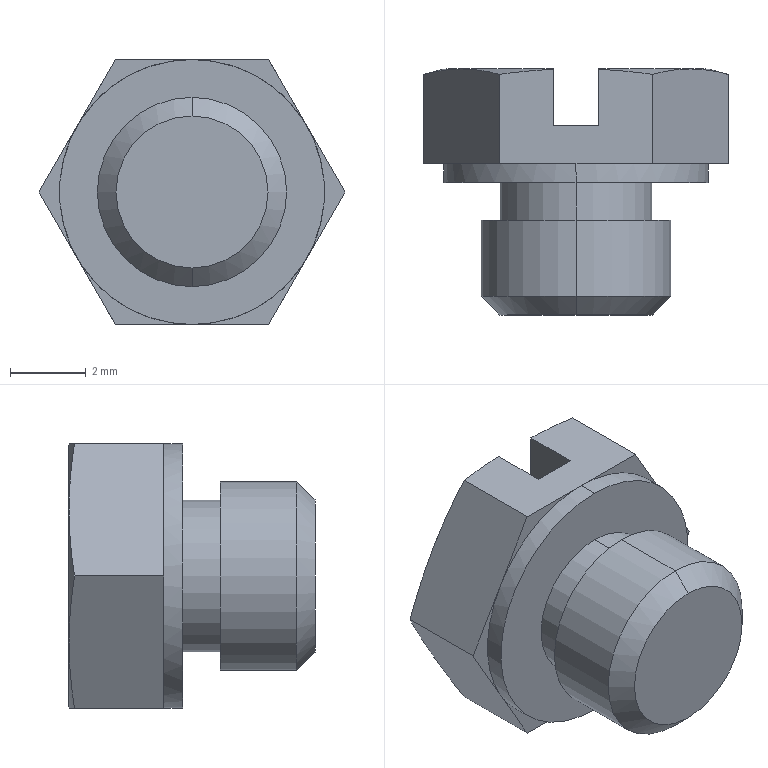Part | SolidWorks | features BaseBody 1 | 1 solid | 34 faces | box 8.083 x 6.5 x 7 mm | volume 172.442 mm3 | plane 18 | cone 8 | cylinder 6 | spline 2 | commonest cylinder face diameters 4 x2 5 x2 7 x2
STEP:
#1=CARTESIAN_POINT('',(0.,3.5,3.5));
#2=VERTEX_POINT('',#1);
#3=CARTESIAN_POINT('',(0.,3.5,-3.5));
#4=VERTEX_POINT('',#3);
#5=CARTESIAN_POINT('',(0.,3.5,0.));
#6=DIRECTION('',(0.,1.,0.));
#7=DIRECTION('',(0.,0.,1.));
#8=AXIS2_PLACEMENT_3D('',#5,#6,#7);
#9=CIRCLE('',#8,3.5);
#10=EDGE_CURVE('',#2,#4,#9,.T.);
#11=ORIENTED_EDGE('',*,*,#10,.T.);
#12=CARTESIAN_POINT('',(0.,4.,-3.5));
#13=VERTEX_POINT('',#12);
#14=CARTESIAN_POINT('',(0.,4.,-3.5));
#15=DIRECTION('',(0.,1.,0.));
#16=VECTOR('',#15,1000.);
#17=LINE('',#14,#16);
#18=EDGE_CURVE('',#4,#13,#17,.T.);
#19=ORIENTED_EDGE('',*,*,#18,.T.);
#20=CARTESIAN_POINT('',(3.031,4.,-1.751));
#21=VERTEX_POINT('',#20);
#22=CARTESIAN_POINT('',(0.,4.,0.));
#23=DIRECTION('',(0.,-1.,0.));
#24=DIRECTION('',(0.,0.,1.));
#25=AXIS2_PLACEMENT_3D('',#22,#23,#24);
#26=CIRCLE('',#25,3.5);
#27=EDGE_CURVE('',#13,#21,#26,.T.);
#28=ORIENTED_EDGE('',*,*,#27,.T.);
#29=CARTESIAN_POINT('',(3.031,4.,1.75));
#30=VERTEX_POINT('',#29);
#31=CARTESIAN_POINT('',(0.,4.,0.));
#32=DIRECTION('',(0.,-1.,0.));
#33=DIRECTION('',(0.,0.,1.));
#34=AXIS2_PLACEMENT_3D('',#31,#32,#33);
#35=CIRCLE('',#34,3.5);
#36=EDGE_CURVE('',#21,#30,#35,.T.);
#37=ORIENTED_EDGE('',*,*,#36,.T.);
#38=CARTESIAN_POINT('',(0.,4.,3.5));
#39=VERTEX_POINT('',#38);
#40=CARTESIAN_POINT('',(0.,4.,0.));
#41=DIRECTION('',(0.,-1.,0.));
#42=DIRECTION('',(0.,0.,1.));
#43=AXIS2_PLACEMENT_3D('',#40,#41,#42);
#44=CIRCLE('',#43,3.5);
#45=EDGE_CURVE('',#30,#39,#44,.T.);
#46=ORIENTED_EDGE('',*,*,#45,.T.);
#47=CARTESIAN_POINT('',(0.,4.,3.5));
#48=DIRECTION('',(0.,1.,0.));
#49=VECTOR('',#48,1000.);
#50=LINE('',#47,#49);
#51=EDGE_CURVE('',#2,#39,#50,.T.);
#52=ORIENTED_EDGE('',*,*,#51,.F.);
#53=EDGE_LOOP('',(#11,#19,#28,#37,#46,#52));
#54=FACE_OUTER_BOUND('',#53,.T.);
#55=CARTESIAN_POINT('',(0.,4.,0.));
#56=DIRECTION('',(0.,1.,0.));
#57=DIRECTION('',(0.,0.,1.));
#58=AXIS2_PLACEMENT_3D('',#55,#56,#57);
#59=CYLINDRICAL_SURFACE('',#58,3.5);
#60=ADVANCED_FACE('',(#54),#59,.T.);
#61=CARTESIAN_POINT('',(0.,2.5,2.));
#62=VERTEX_POINT('',#61);
#63=CARTESIAN_POINT('',(0.,2.5,-2.));
#64=VERTEX_POINT('',#63);
#65=CARTESIAN_POINT('',(0.,2.5,0.));
#66=DIRECTION('',(0.,1.,0.));
#67=DIRECTION('',(0.,0.,1.));
#68=AXIS2_PLACEMENT_3D('',#65,#66,#67);
#69=CIRCLE('',#68,2.);
#70=EDGE_CURVE('',#62,#64,#69,.T.);
#71=ORIENTED_EDGE('',*,*,#70,.T.);
#72=CARTESIAN_POINT('',(0.,3.5,-2.));
#73=VERTEX_POINT('',#72);
#74=CARTESIAN_POINT('',(0.,3.5,-2.));
#75=DIRECTION('',(0.,1.,0.));
#76=VECTOR('',#75,1000.);
#77=LINE('',#74,#76);
#78=EDGE_CURVE('',#64,#73,#77,.T.);
#79=ORIENTED_EDGE('',*,*,#78,.T.);
#80=CARTESIAN_POINT('',(0.,3.5,2.));
#81=VERTEX_POINT('',#80);
#82=CARTESIAN_POINT('',(0.,3.5,0.));
#83=DIRECTION('',(0.,1.,0.));
#84=DIRECTION('',(0.,0.,1.));
#85=AXIS2_PLACEMENT_3D('',#82,#83,#84);
#86=CIRCLE('',#85,2.);
#87=EDGE_CURVE('',#81,#73,#86,.T.);
#88=ORIENTED_EDGE('',*,*,#87,.F.);
#89=CARTESIAN_POINT('',(0.,3.5,2.));
#90=DIRECTION('',(0.,1.,0.));
#91=VECTOR('',#90,1000.);
#92=LINE('',#89,#91);
#93=EDGE_CURVE('',#62,#81,#92,.T.);
#94=ORIENTED_EDGE('',*,*,#93,.F.);
#95=EDGE_LOOP('',(#71,#79,#88,#94));
#96=FACE_OUTER_BOUND('',#95,.T.);
#97=CARTESIAN_POINT('',(0.,3.5,0.));
#98=DIRECTION('',(0.,1.,0.));
#99=DIRECTION('',(0.,0.,1.));
#100=AXIS2_PLACEMENT_3D('',#97,#98,#99);
#101=CYLINDRICAL_SURFACE('',#100,2.);
#102=ADVANCED_FACE('',(#96),#101,.T.);
#103=CARTESIAN_POINT('',(0.,0.4905,2.5));
#104=VERTEX_POINT('',#103);
#105=CARTESIAN_POINT('',(0.,0.4905,-2.5));
#106=VERTEX_POINT('',#105);
#107=CARTESIAN_POINT('',(0.,0.4905,0.));
#108=DIRECTION('',(0.,1.,0.));
#109=DIRECTION('',(1.,0.,0.));
#110=AXIS2_PLACEMENT_3D('',#107,#108,#109);
#111=CIRCLE('',#110,2.5);
#112=EDGE_CURVE('',#104,#106,#111,.T.);
#113=ORIENTED_EDGE('',*,*,#112,.T.);
#114=CARTESIAN_POINT('',(0.,2.5,-2.5));
#115=VERTEX_POINT('',#114);
#116=CARTESIAN_POINT('',(0.,2.5,-2.5));
#117=DIRECTION('',(0.,1.,0.));
#118=VECTOR('',#117,1000.);
#119=LINE('',#116,#118);
#120=EDGE_CURVE('',#106,#115,#119,.T.);
#121=ORIENTED_EDGE('',*,*,#120,.T.);
#122=CARTESIAN_POINT('',(0.,2.5,2.5));
#123=VERTEX_POINT('',#122);
#124=CARTESIAN_POINT('',(0.,2.5,0.));
#125=DIRECTION('',(0.,1.,0.));
#126=DIRECTION('',(0.,0.,1.));
#127=AXIS2_PLACEMENT_3D('',#124,#125,#126);
#128=CIRCLE('',#127,2.5);
#129=EDGE_CURVE('',#123,#115,#128,.T.);
#130=ORIENTED_EDGE('',*,*,#129,.F.);
#131=CARTESIAN_POINT('',(0.,2.5,2.5));
#132=DIRECTION('',(0.,1.,0.));
#133=VECTOR('',#132,1000.);
#134=LINE('',#131,#133);
#135=EDGE_CURVE('',#104,#123,#134,.T.);
#136=ORIENTED_EDGE('',*,*,#135,.F.);
#137=EDGE_LOOP('',(#113,#121,#130,#136));
#138=FACE_OUTER_BOUND('',#137,.T.);
#139=CARTESIAN_POINT('',(0.,2.5,0.));
#140=DIRECTION('',(0.,1.,0.));
#141=DIRECTION('',(0.,0.,1.));
#142=AXIS2_PLACEMENT_3D('',#139,#140,#141);
#143=CYLINDRICAL_SURFACE('',#142,2.5);
#144=ADVANCED_FACE('',(#138),#143,.T.);
#145=CARTESIAN_POINT('',(0.,0.,2.01));
#146=VERTEX_POINT('',#145);
#147=CARTESIAN_POINT('',(0.,0.,-2.01));
#148=VERTEX_POINT('',#147);
#149=CARTESIAN_POINT('',(0.,0.,0.));
#150=DIRECTION('',(0.,1.,0.));
#151=DIRECTION('',(0.,0.,1.));
#152=AXIS2_PLACEMENT_3D('',#149,#150,#151);
#153=CIRCLE('',#152,2.01);
#154=EDGE_CURVE('',#146,#148,#153,.T.);
#155=ORIENTED_EDGE('',*,*,#154,.T.);
#156=CARTESIAN_POINT('',(0.,0.,-2.01));
#157=DIRECTION('',(0.,0.7071,-0.7071));
#158=VECTOR('',#157,1000.);
#159=LINE('',#156,#158);
#160=EDGE_CURVE('',#148,#106,#159,.T.);
#161=ORIENTED_EDGE('',*,*,#160,.T.);
#162=ORIENTED_EDGE('',*,*,#112,.F.);
#163=CARTESIAN_POINT('',(0.,0.,2.01));
#164=DIRECTION('',(0.,0.7071,0.7071));
#165=VECTOR('',#164,1000.);
#166=LINE('',#163,#165);
#167=EDGE_CURVE('',#146,#104,#166,.T.);
#168=ORIENTED_EDGE('',*,*,#167,.F.);
#169=EDGE_LOOP('',(#155,#161,#162,#168));
#170=FACE_OUTER_BOUND('',#169,.T.);
#171=CARTESIAN_POINT('',(0.,0.,0.));
#172=DIRECTION('',(0.,1.,0.));
#173=DIRECTION('',(0.,0.,1.));
#174=AXIS2_PLACEMENT_3D('',#171,#172,#173);
#175=CONICAL_SURFACE('',#174,2.01,0.7854);
#176=ADVANCED_FACE('',(#170),#175,.T.);
#177=ORIENTED_EDGE('',*,*,#18,.F.);
#178=CARTESIAN_POINT('',(0.,3.5,0.));
#179=DIRECTION('',(0.,1.,0.));
#180=DIRECTION('',(0.,0.,1.));
#181=AXIS2_PLACEMENT_3D('',#178,#179,#180);
#182=CIRCLE('',#181,3.5);
#183=EDGE_CURVE('',#4,#2,#182,.T.);
#184=ORIENTED_EDGE('',*,*,#183,.T.);
#185=ORIENTED_EDGE('',*,*,#51,.T.);
#186=CARTESIAN_POINT('',(-3.031,4.,1.75));
#187=VERTEX_POINT('',#186);
#188=CARTESIAN_POINT('',(0.,4.,0.));
#189=DIRECTION('',(0.,-1.,0.));
#190=DIRECTION('',(0.,0.,1.));
#191=AXIS2_PLACEMENT_3D('',#188,#189,#190);
#192=CIRCLE('',#191,3.5);
#193=EDGE_CURVE('',#39,#187,#192,.T.);
#194=ORIENTED_EDGE('',*,*,#193,.T.);
#195=CARTESIAN_POINT('',(-3.031,4.,-1.751));
#196=VERTEX_POINT('',#195);
#197=CARTESIAN_POINT('',(0.,4.,0.));
#198=DIRECTION('',(0.,-1.,0.));
#199=DIRECTION('',(0.,0.,1.));
#200=AXIS2_PLACEMENT_3D('',#197,#198,#199);
#201=CIRCLE('',#200,3.5);
#202=EDGE_CURVE('',#187,#196,#201,.T.);
#203=ORIENTED_EDGE('',*,*,#202,.T.);
#204=CARTESIAN_POINT('',(0.,4.,0.));
#205=DIRECTION('',(0.,-1.,0.));
#206=DIRECTION('',(0.,0.,1.));
#207=AXIS2_PLACEMENT_3D('',#204,#205,#206);
#208=CIRCLE('',#207,3.5);
#209=EDGE_CURVE('',#196,#13,#208,.T.);
#210=ORIENTED_EDGE('',*,*,#209,.T.);
#211=EDGE_LOOP('',(#177,#184,#185,#194,#203,#210));
#212=FACE_OUTER_BOUND('',#211,.T.);
#213=CARTESIAN_POINT('',(0.,4.,0.));
#214=DIRECTION('',(0.,1.,0.));
#215=DIRECTION('',(0.,0.,1.));
#216=AXIS2_PLACEMENT_3D('',#213,#214,#215);
#217=CYLINDRICAL_SURFACE('',#216,3.5);
#218=ADVANCED_FACE('',(#212),#217,.T.);
#219=ORIENTED_EDGE('',*,*,#36,.F.);
#220=CARTESIAN_POINT('',(4.041,4.,0.000000167));
#221=VERTEX_POINT('',#220);
#222=CARTESIAN_POINT('',(3.031,4.,-1.751));
#223=CARTESIAN_POINT('',(3.368,4.,-1.167));
#224=CARTESIAN_POINT('',(3.705,4.,-0.5833));
#225=CARTESIAN_POINT('',(4.041,4.,0.000000167));
#226=B_SPLINE_CURVE_WITH_KNOTS('',3,(#222,#223,#224,#225),.UNSPECIFIED.,.F.,.F.,(4,4),(0.,1.),.UNSPECIFIED.);
#227=EDGE_CURVE('',#21,#221,#226,.T.);
#228=ORIENTED_EDGE('',*,*,#227,.T.);
#229=CARTESIAN_POINT('',(4.041,4.,0.000000167));
#230=CARTESIAN_POINT('',(3.705,4.,0.5833));
#231=CARTESIAN_POINT('',(3.368,4.,1.167));
#232=CARTESIAN_POINT('',(3.031,4.,1.75));
#233=B_SPLINE_CURVE_WITH_KNOTS('',3,(#229,#230,#231,#232),.UNSPECIFIED.,.F.,.F.,(4,4),(0.000000143,1.),.UNSPECIFIED.);
#234=EDGE_CURVE('',#221,#30,#233,.T.);
#235=ORIENTED_EDGE('',*,*,#234,.T.);
#236=EDGE_LOOP('',(#219,#228,#235));
#237=FACE_OUTER_BOUND('',#236,.T.);
#238=CARTESIAN_POINT('',(4.048,4.,1.771));
#239=CARTESIAN_POINT('',(4.048,4.,-1.771));
#240=CARTESIAN_POINT('',(4.041,4.,1.771));
#241=CARTESIAN_POINT('',(4.041,4.,-1.771));
#242=CARTESIAN_POINT('',(3.031,4.,1.771));
#243=CARTESIAN_POINT('',(3.031,4.,-1.771));
#244=B_SPLINE_SURFACE_WITH_KNOTS('',1,1,((#238,#239),(#240,#241),(#242,#243)),.UNSPECIFIED.,.F.,.F.,.F.,(2,1,2),(2,2),(-0.006,0.,1.),(0.,1.),.UNSPECIFIED.);
#245=ADVANCED_FACE('',(#237),#244,.T.);
#246=ORIENTED_EDGE('',*,*,#27,.F.);
#247=CARTESIAN_POINT('',(2.021,4.,-3.5));
#248=VERTEX_POINT('',#247);
#249=CARTESIAN_POINT('',(1.516,4.,-3.5));
#250=DIRECTION('',(1.,0.,0.));
#251=VECTOR('',#250,1000.);
#252=LINE('',#249,#251);
#253=EDGE_CURVE('',#13,#248,#252,.T.);
#254=ORIENTED_EDGE('',*,*,#253,.T.);
#255=CARTESIAN_POINT('',(2.021,4.,-3.5));
#256=CARTESIAN_POINT('',(2.357,4.,-2.917));
#257=CARTESIAN_POINT('',(2.694,4.,-2.334));
#258=CARTESIAN_POINT('',(3.031,4.,-1.751));
#259=B_SPLINE_CURVE_WITH_KNOTS('',3,(#255,#256,#257,#258),.UNSPECIFIED.,.F.,.F.,(4,4),(0.,0.9994),.UNSPECIFIED.);
#260=EDGE_CURVE('',#248,#21,#259,.T.);
#261=ORIENTED_EDGE('',*,*,#260,.T.);
#262=EDGE_LOOP('',(#246,#254,#261));
#263=FACE_OUTER_BOUND('',#262,.T.);
#264=CARTESIAN_POINT('',(3.031,4.,-1.741));
#265=DIRECTION('',(0.,-1.,0.));
#266=DIRECTION('',(-1.,0.,0.));
#267=AXIS2_PLACEMENT_3D('',#264,#265,#266);
#268=PLANE('',#267);
#269=ADVANCED_FACE('',(#263),#268,.T.);
#270=CARTESIAN_POINT('',(-2.021,4.,-3.5));
#271=VERTEX_POINT('',#270);
#272=CARTESIAN_POINT('',(-1.516,4.,-3.5));
#273=DIRECTION('',(1.,0.,0.));
#274=VECTOR('',#273,1000.);
#275=LINE('',#272,#274);
#276=EDGE_CURVE('',#271,#13,#275,.T.);
#277=ORIENTED_EDGE('',*,*,#276,.T.);
#278=ORIENTED_EDGE('',*,*,#209,.F.);
#279=CARTESIAN_POINT('',(-3.031,4.,-1.751));
#280=CARTESIAN_POINT('',(-2.694,4.,-2.334));
#281=CARTESIAN_POINT('',(-2.357,4.,-2.917));
#282=CARTESIAN_POINT('',(-2.021,4.,-3.5));
#283=B_SPLINE_CURVE_WITH_KNOTS('',3,(#279,#280,#281,#282),.UNSPECIFIED.,.F.,.F.,(4,4),(0.0006199,1.),.UNSPECIFIED.);
#284=EDGE_CURVE('',#196,#271,#283,.T.);
#285=ORIENTED_EDGE('',*,*,#284,.T.);
#286=EDGE_LOOP('',(#277,#278,#285));
#287=FACE_OUTER_BOUND('',#286,.T.);
#288=CARTESIAN_POINT('',(0.,4.,-1.741));
#289=DIRECTION('',(0.,-1.,0.));
#290=DIRECTION('',(-1.,0.,0.));
#291=AXIS2_PLACEMENT_3D('',#288,#289,#290);
#292=PLANE('',#291);
#293=ADVANCED_FACE('',(#287),#292,.T.);
#294=ORIENTED_EDGE('',*,*,#202,.F.);
#295=CARTESIAN_POINT('',(-4.041,4.,0.000000167));
#296=VERTEX_POINT('',#295);
#297=CARTESIAN_POINT('',(-3.031,4.,1.75));
#298=CARTESIAN_POINT('',(-3.368,4.,1.167));
#299=CARTESIAN_POINT('',(-3.705,4.,0.5833));
#300=CARTESIAN_POINT('',(-4.041,4.,0.000000167));
#301=B_SPLINE_CURVE_WITH_KNOTS('',3,(#297,#298,#299,#300),.UNSPECIFIED.,.F.,.F.,(4,4),(0.,1.),.UNSPECIFIED.);
#302=EDGE_CURVE('',#187,#296,#301,.T.);
#303=ORIENTED_EDGE('',*,*,#302,.T.);
#304=CARTESIAN_POINT('',(-4.041,4.,0.000000167));
#305=CARTESIAN_POINT('',(-3.705,4.,-0.5833));
#306=CARTESIAN_POINT('',(-3.368,4.,-1.167));
#307=CARTESIAN_POINT('',(-3.031,4.,-1.751));
#308=B_SPLINE_CURVE_WITH_KNOTS('',3,(#304,#305,#306,#307),.UNSPECIFIED.,.F.,.F.,(4,4),(-0.000000071,1.),.UNSPECIFIED.);
#309=EDGE_CURVE('',#296,#196,#308,.T.);
#310=ORIENTED_EDGE('',*,*,#309,.T.);
#311=EDGE_LOOP('',(#294,#303,#310));
#312=FACE_OUTER_BOUND('',#311,.T.);
#313=CARTESIAN_POINT('',(-3.031,4.,1.771));
#314=CARTESIAN_POINT('',(-3.031,4.,-1.771));
#315=CARTESIAN_POINT('',(-4.041,4.,1.771));
#316=CARTESIAN_POINT('',(-4.041,4.,-1.771));
#317=CARTESIAN_POINT('',(-4.048,4.,1.771));
#318=CARTESIAN_POINT('',(-4.048,4.,-1.771));
#319=B_SPLINE_SURFACE_WITH_KNOTS('',1,1,((#313,#314),(#315,#316),(#317,#318)),.UNSPECIFIED.,.F.,.F.,.F.,(2,1,2),(2,2),(0.,1.,1.006),(0.,1.),.UNSPECIFIED.);
#320=ADVANCED_FACE('',(#312),#319,.T.);
#321=ORIENTED_EDGE('',*,*,#87,.T.);
#322=CARTESIAN_POINT('',(0.,3.5,0.));
#323=DIRECTION('',(0.,1.,0.));
#324=DIRECTION('',(0.,0.,1.));
#325=AXIS2_PLACEMENT_3D('',#322,#323,#324);
#326=CIRCLE('',#325,2.);
#327=EDGE_CURVE('',#73,#81,#326,.T.);
#328=ORIENTED_EDGE('',*,*,#327,.T.);
#329=EDGE_LOOP('',(#321,#328));
#330=FACE_BOUND('',#329,.T.);
#331=ORIENTED_EDGE('',*,*,#10,.F.);
#332=ORIENTED_EDGE('',*,*,#183,.F.);
#333=EDGE_LOOP('',(#331,#332));
#334=FACE_OUTER_BOUND('',#333,.T.);
#335=CARTESIAN_POINT('',(3.5,3.5,3.542));
#336=DIRECTION('',(0.,-1.,0.));
#337=DIRECTION('',(-1.,0.,0.));
#338=AXIS2_PLACEMENT_3D('',#335,#336,#337);
#339=PLANE('',#338);
#340=ADVANCED_FACE('',(#330,#334),#339,.T.);
#341=CARTESIAN_POINT('',(2.021,6.355,-3.5));
#342=VERTEX_POINT('',#341);
#343=CARTESIAN_POINT('',(2.021,6.5,-3.5));
#344=DIRECTION('',(0.,1.,0.));
#345=VECTOR('',#344,1000.);
#346=LINE('',#343,#345);
#347=EDGE_CURVE('',#248,#342,#346,.T.);
#348=ORIENTED_EDGE('',*,*,#347,.T.);
#349=CARTESIAN_POINT('',(3.031,6.5,-1.75));
#350=VERTEX_POINT('',#349);
#351=CARTESIAN_POINT('',(2.021,6.355,-3.5));
#352=CARTESIAN_POINT('',(2.356,6.445,-2.919));
#353=CARTESIAN_POINT('',(2.693,6.5,-2.336));
#354=CARTESIAN_POINT('',(3.031,6.5,-1.75));
#355=B_SPLINE_CURVE_WITH_KNOTS('',3,(#351,#352,#353,#354),.UNSPECIFIED.,.F.,.F.,(4,4),(0.,0.002026),.UNSPECIFIED.);
#356=EDGE_CURVE('',#342,#350,#355,.T.);
#357=ORIENTED_EDGE('',*,*,#356,.T.);
#358=CARTESIAN_POINT('',(4.041,6.355,0.));
#359=VERTEX_POINT('',#358);
#360=CARTESIAN_POINT('',(3.031,6.5,-1.75));
#361=CARTESIAN_POINT('',(3.37,6.5,-1.164));
#362=CARTESIAN_POINT('',(3.706,6.445,-0.5808));
#363=CARTESIAN_POINT('',(4.041,6.355,0.));
#364=B_SPLINE_CURVE_WITH_KNOTS('',3,(#360,#361,#362,#363),.UNSPECIFIED.,.F.,.F.,(4,4),(0.,0.002026),.UNSPECIFIED.);
#365=EDGE_CURVE('',#350,#359,#364,.T.);
#366=ORIENTED_EDGE('',*,*,#365,.T.);
#367=CARTESIAN_POINT('',(4.041,6.5,0.));
#368=DIRECTION('',(0.,-1.,0.));
#369=VECTOR('',#368,1000.);
#370=LINE('',#367,#369);
#371=EDGE_CURVE('',#359,#221,#370,.T.);
#372=ORIENTED_EDGE('',*,*,#371,.T.);
#373=ORIENTED_EDGE('',*,*,#227,.F.);
#374=ORIENTED_EDGE('',*,*,#260,.F.);
#375=EDGE_LOOP('',(#348,#357,#366,#372,#373,#374));
#376=FACE_OUTER_BOUND('',#375,.T.);
#377=CARTESIAN_POINT('',(2.021,6.515,-3.5));
#378=DIRECTION('',(0.866,0.,-0.5));
#379=DIRECTION('',(0.5,0.,0.866));
#380=AXIS2_PLACEMENT_3D('',#377,#378,#379);
#381=PLANE('',#380);
#382=ADVANCED_FACE('',(#376),#381,.T.);
#383=ORIENTED_EDGE('',*,*,#234,.F.);
#384=ORIENTED_EDGE('',*,*,#371,.F.);
#385=CARTESIAN_POINT('',(3.031,6.5,1.75));
#386=VERTEX_POINT('',#385);
#387=CARTESIAN_POINT('',(4.041,6.355,0.));
#388=CARTESIAN_POINT('',(3.706,6.445,0.5808));
#389=CARTESIAN_POINT('',(3.37,6.5,1.164));
#390=CARTESIAN_POINT('',(3.031,6.5,1.75));
#391=B_SPLINE_CURVE_WITH_KNOTS('',3,(#387,#388,#389,#390),.UNSPECIFIED.,.F.,.F.,(4,4),(0.,0.002026),.UNSPECIFIED.);
#392=EDGE_CURVE('',#359,#386,#391,.T.);
#393=ORIENTED_EDGE('',*,*,#392,.T.);
#394=CARTESIAN_POINT('',(2.021,6.355,3.5));
#395=VERTEX_POINT('',#394);
#396=CARTESIAN_POINT('',(3.031,6.5,1.75));
#397=CARTESIAN_POINT('',(2.693,6.5,2.336));
#398=CARTESIAN_POINT('',(2.356,6.445,2.919));
#399=CARTESIAN_POINT('',(2.021,6.355,3.5));
#400=B_SPLINE_CURVE_WITH_KNOTS('',3,(#396,#397,#398,#399),.UNSPECIFIED.,.F.,.F.,(4,4),(0.,0.002026),.UNSPECIFIED.);
#401=EDGE_CURVE('',#386,#395,#400,.T.);
#402=ORIENTED_EDGE('',*,*,#401,.T.);
#403=CARTESIAN_POINT('',(2.021,4.,3.5));
#404=VERTEX_POINT('',#403);
#405=CARTESIAN_POINT('',(2.021,6.5,3.5));
#406=DIRECTION('',(0.,-1.,0.));
#407=VECTOR('',#406,1000.);
#408=LINE('',#405,#407);
#409=EDGE_CURVE('',#395,#404,#408,.T.);
#410=ORIENTED_EDGE('',*,*,#409,.T.);
#411=CARTESIAN_POINT('',(3.031,4.,1.75));
#412=DIRECTION('',(0.5,0.,-0.866));
#413=VECTOR('',#412,1000.);
#414=LINE('',#411,#413);
#415=EDGE_CURVE('',#404,#30,#414,.T.);
#416=ORIENTED_EDGE('',*,*,#415,.T.);
#417=EDGE_LOOP('',(#383,#384,#393,#402,#410,#416));
#418=FACE_OUTER_BOUND('',#417,.T.);
#419=CARTESIAN_POINT('',(4.041,6.515,0.));
#420=DIRECTION('',(0.866,0.,0.5));
#421=DIRECTION('',(-0.5,0.,0.866));
#422=AXIS2_PLACEMENT_3D('',#419,#420,#421);
#423=PLANE('',#422);
#424=ADVANCED_FACE('',(#418),#423,.T.);
#425=CARTESIAN_POINT('',(-0.6,5.,-3.5));
#426=VERTEX_POINT('',#425);
#427=CARTESIAN_POINT('',(-0.6,6.486,-3.5));
#428=VERTEX_POINT('',#427);
#429=CARTESIAN_POINT('',(-0.6,6.5,-3.5));
#430=DIRECTION('',(0.,1.,0.));
#431=VECTOR('',#430,1000.);
#432=LINE('',#429,#431);
#433=EDGE_CURVE('',#426,#428,#432,.T.);
#434=ORIENTED_EDGE('',*,*,#433,.F.);
#435=CARTESIAN_POINT('',(0.6,5.,-3.5));
#436=VERTEX_POINT('',#435);
#437=CARTESIAN_POINT('',(-0.6,5.,-3.5));
#438=DIRECTION('',(-1.,0.,0.));
#439=VECTOR('',#438,1000.);
#440=LINE('',#437,#439);
#441=EDGE_CURVE('',#436,#426,#440,.T.);
#442=ORIENTED_EDGE('',*,*,#441,.F.);
#443=CARTESIAN_POINT('',(0.6,6.486,-3.5));
#444=VERTEX_POINT('',#443);
#445=CARTESIAN_POINT('',(0.6,6.5,-3.5));
#446=DIRECTION('',(0.,-1.,0.));
#447=VECTOR('',#446,1000.);
#448=LINE('',#445,#447);
#449=EDGE_CURVE('',#444,#436,#448,.T.);
#450=ORIENTED_EDGE('',*,*,#449,.F.);
#451=CARTESIAN_POINT('',(0.6,6.486,-3.5));
#452=CARTESIAN_POINT('',(1.076,6.465,-3.5));
#453=CARTESIAN_POINT('',(1.549,6.418,-3.5));
#454=CARTESIAN_POINT('',(2.021,6.355,-3.5));
#455=B_SPLINE_CURVE_WITH_KNOTS('',3,(#451,#452,#453,#454),.UNSPECIFIED.,.F.,.F.,(4,4),(0.,0.001427),.UNSPECIFIED.);
#456=EDGE_CURVE('',#444,#342,#455,.T.);
#457=ORIENTED_EDGE('',*,*,#456,.T.);
#458=ORIENTED_EDGE('',*,*,#347,.F.);
#459=ORIENTED_EDGE('',*,*,#253,.F.);
#460=ORIENTED_EDGE('',*,*,#276,.F.);
#461=CARTESIAN_POINT('',(-2.021,6.355,-3.5));
#462=VERTEX_POINT('',#461);
#463=CARTESIAN_POINT('',(-2.021,6.486,-3.5));
#464=DIRECTION('',(0.,1.,0.));
#465=VECTOR('',#464,1000.);
#466=LINE('',#463,#465);
#467=EDGE_CURVE('',#271,#462,#466,.T.);
#468=ORIENTED_EDGE('',*,*,#467,.T.);
#469=CARTESIAN_POINT('',(-0.6,6.486,-3.5));
#470=CARTESIAN_POINT('',(-1.076,6.465,-3.5));
#471=CARTESIAN_POINT('',(-1.549,6.418,-3.5));
#472=CARTESIAN_POINT('',(-2.021,6.355,-3.5));
#473=B_SPLINE_CURVE_WITH_KNOTS('',3,(#469,#470,#471,#472),.UNSPECIFIED.,.F.,.F.,(4,4),(0.,0.001427),.UNSPECIFIED.);
#474=EDGE_CURVE('',#428,#462,#473,.T.);
#475=ORIENTED_EDGE('',*,*,#474,.F.);
#476=EDGE_LOOP('',(#434,#442,#450,#457,#458,#459,#460,#468,#475));
#477=FACE_OUTER_BOUND('',#476,.T.);
#478=CARTESIAN_POINT('',(-2.021,6.501,-3.5));
#479=DIRECTION('',(0.,0.,-1.));
#480=DIRECTION('',(1.,0.,0.));
#481=AXIS2_PLACEMENT_3D('',#478,#479,#480);
#482=PLANE('',#481);
#483=ADVANCED_FACE('',(#477),#482,.T.);
#484=CARTESIAN_POINT('',(-4.041,6.355,0.));
#485=VERTEX_POINT('',#484);
#486=CARTESIAN_POINT('',(-4.041,6.5,0.));
#487=DIRECTION('',(0.,1.,0.));
#488=VECTOR('',#487,1000.);
#489=LINE('',#486,#488);
#490=EDGE_CURVE('',#296,#485,#489,.T.);
#491=ORIENTED_EDGE('',*,*,#490,.T.);
#492=CARTESIAN_POINT('',(-3.031,6.5,-1.75));
#493=VERTEX_POINT('',#492);
#494=CARTESIAN_POINT('',(-4.041,6.355,0.));
#495=CARTESIAN_POINT('',(-3.706,6.445,-0.5808));
#496=CARTESIAN_POINT('',(-3.37,6.5,-1.164));
#497=CARTESIAN_POINT('',(-3.031,6.5,-1.75));
#498=B_SPLINE_CURVE_WITH_KNOTS('',3,(#494,#495,#496,#497),.UNSPECIFIED.,.F.,.F.,(4,4),(0.,0.002026),.UNSPECIFIED.);
#499=EDGE_CURVE('',#485,#493,#498,.T.);
#500=ORIENTED_EDGE('',*,*,#499,.T.);
#501=CARTESIAN_POINT('',(-3.031,6.5,-1.75));
#502=CARTESIAN_POINT('',(-2.693,6.5,-2.336));
#503=CARTESIAN_POINT('',(-2.356,6.445,-2.919));
#504=CARTESIAN_POINT('',(-2.021,6.355,-3.5));
#505=B_SPLINE_CURVE_WITH_KNOTS('',3,(#501,#502,#503,#504),.UNSPECIFIED.,.F.,.F.,(4,4),(0.,0.002026),.UNSPECIFIED.);
#506=EDGE_CURVE('',#493,#462,#505,.T.);
#507=ORIENTED_EDGE('',*,*,#506,.T.);
#508=ORIENTED_EDGE('',*,*,#467,.F.);
#509=ORIENTED_EDGE('',*,*,#284,.F.);
#510=ORIENTED_EDGE('',*,*,#309,.F.);
#511=EDGE_LOOP('',(#491,#500,#507,#508,#509,#510));
#512=FACE_OUTER_BOUND('',#511,.T.);
#513=CARTESIAN_POINT('',(-4.041,6.515,0.));
#514=DIRECTION('',(-0.866,0.,-0.5));
#515=DIRECTION('',(0.5,0.,-0.866));
#516=AXIS2_PLACEMENT_3D('',#513,#514,#515);
#517=PLANE('',#516);
#518=ADVANCED_FACE('',(#512),#517,.T.);
#519=CARTESIAN_POINT('',(-2.021,4.,3.5));
#520=VERTEX_POINT('',#519);
#521=CARTESIAN_POINT('',(-3.031,4.,1.75));
#522=DIRECTION('',(0.5,0.,0.866));
#523=VECTOR('',#522,1000.);
#524=LINE('',#521,#523);
#525=EDGE_CURVE('',#187,#520,#524,.T.);
#526=ORIENTED_EDGE('',*,*,#525,.T.);
#527=CARTESIAN_POINT('',(-2.021,6.355,3.5));
#528=VERTEX_POINT('',#527);
#529=CARTESIAN_POINT('',(-2.021,6.5,3.5));
#530=DIRECTION('',(0.,1.,0.));
#531=VECTOR('',#530,1000.);
#532=LINE('',#529,#531);
#533=EDGE_CURVE('',#520,#528,#532,.T.);
#534=ORIENTED_EDGE('',*,*,#533,.T.);
#535=CARTESIAN_POINT('',(-3.031,6.5,1.75));
#536=VERTEX_POINT('',#535);
#537=CARTESIAN_POINT('',(-2.021,6.355,3.5));
#538=CARTESIAN_POINT('',(-2.356,6.445,2.919));
#539=CARTESIAN_POINT('',(-2.693,6.5,2.336));
#540=CARTESIAN_POINT('',(-3.031,6.5,1.75));
#541=B_SPLINE_CURVE_WITH_KNOTS('',3,(#537,#538,#539,#540),.UNSPECIFIED.,.F.,.F.,(4,4),(0.,0.002026),.UNSPECIFIED.);
#542=EDGE_CURVE('',#528,#536,#541,.T.);
#543=ORIENTED_EDGE('',*,*,#542,.T.);
#544=CARTESIAN_POINT('',(-3.031,6.5,1.75));
#545=CARTESIAN_POINT('',(-3.37,6.5,1.164));
#546=CARTESIAN_POINT('',(-3.706,6.445,0.5808));
#547=CARTESIAN_POINT('',(-4.041,6.355,0.));
#548=B_SPLINE_CURVE_WITH_KNOTS('',3,(#544,#545,#546,#547),.UNSPECIFIED.,.F.,.F.,(4,4),(0.,0.002026),.UNSPECIFIED.);
#549=EDGE_CURVE('',#536,#485,#548,.T.);
#550=ORIENTED_EDGE('',*,*,#549,.T.);
#551=ORIENTED_EDGE('',*,*,#490,.F.);
#552=ORIENTED_EDGE('',*,*,#302,.F.);
#553=EDGE_LOOP('',(#526,#534,#543,#550,#551,#552));
#554=FACE_OUTER_BOUND('',#553,.T.);
#555=CARTESIAN_POINT('',(-2.021,6.515,3.5));
#556=DIRECTION('',(-0.866,0.,0.5));
#557=DIRECTION('',(-0.5,0.,-0.866));
#558=AXIS2_PLACEMENT_3D('',#555,#556,#557);
#559=PLANE('',#558);
#560=ADVANCED_FACE('',(#554),#559,.T.);
#561=ORIENTED_EDGE('',*,*,#78,.F.);
#562=CARTESIAN_POINT('',(0.,2.5,0.));
#563=DIRECTION('',(0.,1.,0.));
#564=DIRECTION('',(0.,0.,1.));
#565=AXIS2_PLACEMENT_3D('',#562,#563,#564);
#566=CIRCLE('',#565,2.);
#567=EDGE_CURVE('',#64,#62,#566,.T.);
#568=ORIENTED_EDGE('',*,*,#567,.T.);
#569=ORIENTED_EDGE('',*,*,#93,.T.);
#570=ORIENTED_EDGE('',*,*,#327,.F.);
#571=EDGE_LOOP('',(#561,#568,#569,#570));
#572=FACE_OUTER_BOUND('',#571,.T.);
#573=CARTESIAN_POINT('',(0.,3.5,0.));
#574=DIRECTION('',(0.,1.,0.));
#575=DIRECTION('',(0.,0.,1.));
#576=AXIS2_PLACEMENT_3D('',#573,#574,#575);
#577=CYLINDRICAL_SURFACE('',#576,2.);
#578=ADVANCED_FACE('',(#572),#577,.T.);
#579=ORIENTED_EDGE('',*,*,#356,.F.);
#580=ORIENTED_EDGE('',*,*,#456,.F.);
#581=CARTESIAN_POINT('',(0.6,6.5,-3.448));
#582=VERTEX_POINT('',#581);
#583=CARTESIAN_POINT('',(0.6,6.5,-3.448));
#584=DIRECTION('',(0.,-0.2553,-0.9669));
#585=VECTOR('',#584,1000.);
#586=LINE('',#583,#585);
#587=EDGE_CURVE('',#582,#444,#586,.T.);
#588=ORIENTED_EDGE('',*,*,#587,.F.);
#589=CARTESIAN_POINT('',(0.,6.5,0.));
#590=DIRECTION('',(0.,-1.,0.));
#591=DIRECTION('',(0.,0.,-1.));
#592=AXIS2_PLACEMENT_3D('',#589,#590,#591);
#593=CIRCLE('',#592,3.5);
#594=EDGE_CURVE('',#582,#350,#593,.T.);
#595=ORIENTED_EDGE('',*,*,#594,.T.);
#596=EDGE_LOOP('',(#579,#580,#588,#595));
#597=FACE_OUTER_BOUND('',#596,.T.);
#598=CARTESIAN_POINT('',(0.,6.5,0.));
#599=DIRECTION('',(0.,-1.,0.));
#600=DIRECTION('',(0.,0.,-1.));
#601=AXIS2_PLACEMENT_3D('',#598,#599,#600);
#602=CONICAL_SURFACE('',#601,3.5,1.309);
#603=ADVANCED_FACE('',(#597),#602,.T.);
#604=ORIENTED_EDGE('',*,*,#365,.F.);
#605=CARTESIAN_POINT('',(0.,6.5,0.));
#606=DIRECTION('',(0.,-1.,0.));
#607=DIRECTION('',(0.,0.,-1.));
#608=AXIS2_PLACEMENT_3D('',#605,#606,#607);
#609=CIRCLE('',#608,3.5);
#610=EDGE_CURVE('',#350,#386,#609,.T.);
#611=ORIENTED_EDGE('',*,*,#610,.T.);
#612=ORIENTED_EDGE('',*,*,#392,.F.);
#613=EDGE_LOOP('',(#604,#611,#612));
#614=FACE_OUTER_BOUND('',#613,.T.);
#615=CARTESIAN_POINT('',(0.,6.5,0.));
#616=DIRECTION('',(0.,-1.,0.));
#617=DIRECTION('',(0.,0.,-1.));
#618=AXIS2_PLACEMENT_3D('',#615,#616,#617);
#619=CONICAL_SURFACE('',#618,3.5,1.309);
#620=ADVANCED_FACE('',(#614),#619,.T.);
#621=ORIENTED_EDGE('',*,*,#525,.F.);
#622=ORIENTED_EDGE('',*,*,#193,.F.);
#623=CARTESIAN_POINT('',(-1.516,4.,3.5));
#624=DIRECTION('',(-1.,0.,0.));
#625=VECTOR('',#624,1000.);
#626=LINE('',#623,#625);
#627=EDGE_CURVE('',#39,#520,#626,.T.);
#628=ORIENTED_EDGE('',*,*,#627,.T.);
#629=EDGE_LOOP('',(#621,#622,#628));
#630=FACE_OUTER_BOUND('',#629,.T.);
#631=CARTESIAN_POINT('',(0.,4.,3.5));
#632=DIRECTION('',(0.,-1.,0.));
#633=DIRECTION('',(-1.,0.,0.));
#634=AXIS2_PLACEMENT_3D('',#631,#632,#633);
#635=PLANE('',#634);
#636=ADVANCED_FACE('',(#630),#635,.T.);
#637=ORIENTED_EDGE('',*,*,#45,.F.);
#638=ORIENTED_EDGE('',*,*,#415,.F.);
#639=CARTESIAN_POINT('',(1.516,4.,3.5));
#640=DIRECTION('',(-1.,0.,0.));
#641=VECTOR('',#640,1000.);
#642=LINE('',#639,#641);
#643=EDGE_CURVE('',#404,#39,#642,.T.);
#644=ORIENTED_EDGE('',*,*,#643,.T.);
#645=EDGE_LOOP('',(#637,#638,#644));
#646=FACE_OUTER_BOUND('',#645,.T.);
#647=CARTESIAN_POINT('',(3.031,4.,3.5));
#648=DIRECTION('',(0.,-1.,0.));
#649=DIRECTION('',(-1.,0.,0.));
#650=AXIS2_PLACEMENT_3D('',#647,#648,#649);
#651=PLANE('',#650);
#652=ADVANCED_FACE('',(#646),#651,.T.);
#653=ORIENTED_EDGE('',*,*,#409,.F.);
#654=CARTESIAN_POINT('',(0.6,6.486,3.5));
#655=VERTEX_POINT('',#654);
#656=CARTESIAN_POINT('',(2.021,6.355,3.5));
#657=CARTESIAN_POINT('',(1.549,6.418,3.5));
#658=CARTESIAN_POINT('',(1.076,6.465,3.5));
#659=CARTESIAN_POINT('',(0.6,6.486,3.5));
#660=B_SPLINE_CURVE_WITH_KNOTS('',3,(#656,#657,#658,#659),.UNSPECIFIED.,.F.,.F.,(4,4),(0.,0.001427),.UNSPECIFIED.);
#661=EDGE_CURVE('',#395,#655,#660,.T.);
#662=ORIENTED_EDGE('',*,*,#661,.T.);
#663=CARTESIAN_POINT('',(0.6,5.,3.5));
#664=VERTEX_POINT('',#663);
#665=CARTESIAN_POINT('',(0.6,6.5,3.5));
#666=DIRECTION('',(0.,1.,0.));
#667=VECTOR('',#666,1000.);
#668=LINE('',#665,#667);
#669=EDGE_CURVE('',#664,#655,#668,.T.);
#670=ORIENTED_EDGE('',*,*,#669,.F.);
#671=CARTESIAN_POINT('',(-0.6,5.,3.5));
#672=VERTEX_POINT('',#671);
#673=CARTESIAN_POINT('',(-0.6,5.,3.5));
#674=DIRECTION('',(1.,0.,0.));
#675=VECTOR('',#674,1000.);
#676=LINE('',#673,#675);
#677=EDGE_CURVE('',#672,#664,#676,.T.);
#678=ORIENTED_EDGE('',*,*,#677,.F.);
#679=CARTESIAN_POINT('',(-0.6,6.486,3.5));
#680=VERTEX_POINT('',#679);
#681=CARTESIAN_POINT('',(-0.6,6.5,3.5));
#682=DIRECTION('',(0.,-1.,0.));
#683=VECTOR('',#682,1000.);
#684=LINE('',#681,#683);
#685=EDGE_CURVE('',#680,#672,#684,.T.);
#686=ORIENTED_EDGE('',*,*,#685,.F.);
#687=CARTESIAN_POINT('',(-0.6,6.486,3.5));
#688=CARTESIAN_POINT('',(-1.076,6.465,3.5));
#689=CARTESIAN_POINT('',(-1.549,6.418,3.5));
#690=CARTESIAN_POINT('',(-2.021,6.355,3.5));
#691=B_SPLINE_CURVE_WITH_KNOTS('',3,(#687,#688,#689,#690),.UNSPECIFIED.,.F.,.F.,(4,4),(0.,0.001427),.UNSPECIFIED.);
#692=EDGE_CURVE('',#680,#528,#691,.T.);
#693=ORIENTED_EDGE('',*,*,#692,.T.);
#694=ORIENTED_EDGE('',*,*,#533,.F.);
#695=ORIENTED_EDGE('',*,*,#627,.F.);
#696=ORIENTED_EDGE('',*,*,#643,.F.);
#697=EDGE_LOOP('',(#653,#662,#670,#678,#686,#693,#694,#695,#696));
#698=FACE_OUTER_BOUND('',#697,.T.);
#699=CARTESIAN_POINT('',(2.021,6.501,3.5));
#700=DIRECTION('',(0.,0.,1.));
#701=DIRECTION('',(-1.,0.,0.));
#702=AXIS2_PLACEMENT_3D('',#699,#700,#701);
#703=PLANE('',#702);
#704=ADVANCED_FACE('',(#698),#703,.T.);
#705=ORIENTED_EDGE('',*,*,#401,.F.);
#706=CARTESIAN_POINT('',(0.6,6.5,3.448));
#707=VERTEX_POINT('',#706);
#708=CARTESIAN_POINT('',(0.,6.5,0.));
#709=DIRECTION('',(0.,-1.,0.));
#710=DIRECTION('',(0.,0.,-1.));
#711=AXIS2_PLACEMENT_3D('',#708,#709,#710);
#712=CIRCLE('',#711,3.5);
#713=EDGE_CURVE('',#386,#707,#712,.T.);
#714=ORIENTED_EDGE('',*,*,#713,.T.);
#715=CARTESIAN_POINT('',(0.6,6.486,3.5));
#716=DIRECTION('',(0.,0.2553,-0.9669));
#717=VECTOR('',#716,1000.);
#718=LINE('',#715,#717);
#719=EDGE_CURVE('',#655,#707,#718,.T.);
#720=ORIENTED_EDGE('',*,*,#719,.F.);
#721=ORIENTED_EDGE('',*,*,#661,.F.);
#722=EDGE_LOOP('',(#705,#714,#720,#721));
#723=FACE_OUTER_BOUND('',#722,.T.);
#724=CARTESIAN_POINT('',(0.,6.5,0.));
#725=DIRECTION('',(0.,-1.,0.));
#726=DIRECTION('',(0.,0.,-1.));
#727=AXIS2_PLACEMENT_3D('',#724,#725,#726);
#728=CONICAL_SURFACE('',#727,3.5,1.309);
#729=ADVANCED_FACE('',(#723),#728,.T.);
#730=CARTESIAN_POINT('',(0.,6.5,0.));
#731=DIRECTION('',(0.,-1.,0.));
#732=DIRECTION('',(0.,0.,-1.));
#733=AXIS2_PLACEMENT_3D('',#730,#731,#732);
#734=CIRCLE('',#733,3.5);
#735=EDGE_CURVE('',#536,#493,#734,.T.);
#736=ORIENTED_EDGE('',*,*,#735,.T.);
#737=ORIENTED_EDGE('',*,*,#499,.F.);
#738=ORIENTED_EDGE('',*,*,#549,.F.);
#739=EDGE_LOOP('',(#736,#737,#738));
#740=FACE_OUTER_BOUND('',#739,.T.);
#741=CARTESIAN_POINT('',(0.,6.5,0.));
#742=DIRECTION('',(0.,-1.,0.));
#743=DIRECTION('',(0.,0.,-1.));
#744=AXIS2_PLACEMENT_3D('',#741,#742,#743);
#745=CONICAL_SURFACE('',#744,3.5,1.309);
#746=ADVANCED_FACE('',(#740),#745,.T.);
#747=ORIENTED_EDGE('',*,*,#506,.F.);
#748=CARTESIAN_POINT('',(-0.6,6.5,-3.448));
#749=VERTEX_POINT('',#748);
#750=CARTESIAN_POINT('',(0.,6.5,0.));
#751=DIRECTION('',(0.,-1.,0.));
#752=DIRECTION('',(0.,0.,-1.));
#753=AXIS2_PLACEMENT_3D('',#750,#751,#752);
#754=CIRCLE('',#753,3.5);
#755=EDGE_CURVE('',#493,#749,#754,.T.);
#756=ORIENTED_EDGE('',*,*,#755,.T.);
#757=CARTESIAN_POINT('',(-0.6,6.486,-3.5));
#758=DIRECTION('',(0.,0.2553,0.9669));
#759=VECTOR('',#758,1000.);
#760=LINE('',#757,#759);
#761=EDGE_CURVE('',#428,#749,#760,.T.);
#762=ORIENTED_EDGE('',*,*,#761,.F.);
#763=ORIENTED_EDGE('',*,*,#474,.T.);
#764=EDGE_LOOP('',(#747,#756,#762,#763));
#765=FACE_OUTER_BOUND('',#764,.T.);
#766=CARTESIAN_POINT('',(0.,6.5,0.));
#767=DIRECTION('',(0.,-1.,0.));
#768=DIRECTION('',(0.,0.,-1.));
#769=AXIS2_PLACEMENT_3D('',#766,#767,#768);
#770=CONICAL_SURFACE('',#769,3.5,1.309);
#771=ADVANCED_FACE('',(#765),#770,.T.);
#772=ORIENTED_EDGE('',*,*,#542,.F.);
#773=ORIENTED_EDGE('',*,*,#692,.F.);
#774=CARTESIAN_POINT('',(-0.6,6.5,3.448));
#775=VERTEX_POINT('',#774);
#776=CARTESIAN_POINT('',(-0.6,6.5,3.448));
#777=DIRECTION('',(0.,-0.2553,0.9669));
#778=VECTOR('',#777,1000.);
#779=LINE('',#776,#778);
#780=EDGE_CURVE('',#775,#680,#779,.T.);
#781=ORIENTED_EDGE('',*,*,#780,.F.);
#782=CARTESIAN_POINT('',(0.,6.5,0.));
#783=DIRECTION('',(0.,-1.,0.));
#784=DIRECTION('',(0.,0.,-1.));
#785=AXIS2_PLACEMENT_3D('',#782,#783,#784);
#786=CIRCLE('',#785,3.5);
#787=EDGE_CURVE('',#775,#536,#786,.T.);
#788=ORIENTED_EDGE('',*,*,#787,.T.);
#789=EDGE_LOOP('',(#772,#773,#781,#788));
#790=FACE_OUTER_BOUND('',#789,.T.);
#791=CARTESIAN_POINT('',(0.,6.5,0.));
#792=DIRECTION('',(0.,-1.,0.));
#793=DIRECTION('',(0.,0.,-1.));
#794=AXIS2_PLACEMENT_3D('',#791,#792,#793);
#795=CONICAL_SURFACE('',#794,3.5,1.309);
#796=ADVANCED_FACE('',(#790),#795,.T.);
#797=ORIENTED_EDGE('',*,*,#70,.F.);
#798=ORIENTED_EDGE('',*,*,#567,.F.);
#799=EDGE_LOOP('',(#797,#798));
#800=FACE_BOUND('',#799,.T.);
#801=ORIENTED_EDGE('',*,*,#129,.T.);
#802=CARTESIAN_POINT('',(0.,2.5,0.));
#803=DIRECTION('',(0.,1.,0.));
#804=DIRECTION('',(0.,0.,1.));
#805=AXIS2_PLACEMENT_3D('',#802,#803,#804);
#806=CIRCLE('',#805,2.5);
#807=EDGE_CURVE('',#115,#123,#806,.T.);
#808=ORIENTED_EDGE('',*,*,#807,.T.);
#809=EDGE_LOOP('',(#801,#808));
#810=FACE_OUTER_BOUND('',#809,.T.);
#811=CARTESIAN_POINT('',(-2.5,2.5,2.53));
#812=DIRECTION('',(0.,1.,0.));
#813=DIRECTION('',(1.,0.,0.));
#814=AXIS2_PLACEMENT_3D('',#811,#812,#813);
#815=PLANE('',#814);
#816=ADVANCED_FACE('',(#800,#810),#815,.T.);
#817=ORIENTED_EDGE('',*,*,#610,.F.);
#818=ORIENTED_EDGE('',*,*,#594,.F.);
#819=CARTESIAN_POINT('',(0.6,6.5,3.448));
#820=DIRECTION('',(0.,0.,1.));
#821=VECTOR('',#820,1000.);
#822=LINE('',#819,#821);
#823=EDGE_CURVE('',#582,#707,#822,.T.);
#824=ORIENTED_EDGE('',*,*,#823,.T.);
#825=ORIENTED_EDGE('',*,*,#713,.F.);
#826=EDGE_LOOP('',(#817,#818,#824,#825));
#827=FACE_OUTER_BOUND('',#826,.T.);
#828=CARTESIAN_POINT('',(0.6,6.5,3.49));
#829=DIRECTION('',(0.,1.,0.));
#830=DIRECTION('',(1.,0.,0.));
#831=AXIS2_PLACEMENT_3D('',#828,#829,#830);
#832=PLANE('',#831);
#833=ADVANCED_FACE('',(#827),#832,.T.);
#834=ORIENTED_EDGE('',*,*,#735,.F.);
#835=ORIENTED_EDGE('',*,*,#787,.F.);
#836=CARTESIAN_POINT('',(-0.6,6.5,3.448));
#837=DIRECTION('',(0.,0.,-1.));
#838=VECTOR('',#837,1000.);
#839=LINE('',#836,#838);
#840=EDGE_CURVE('',#775,#749,#839,.T.);
#841=ORIENTED_EDGE('',*,*,#840,.T.);
#842=ORIENTED_EDGE('',*,*,#755,.F.);
#843=EDGE_LOOP('',(#834,#835,#841,#842));
#844=FACE_OUTER_BOUND('',#843,.T.);
#845=CARTESIAN_POINT('',(-3.5,6.5,3.49));
#846=DIRECTION('',(0.,1.,0.));
#847=DIRECTION('',(1.,0.,0.));
#848=AXIS2_PLACEMENT_3D('',#845,#846,#847);
#849=PLANE('',#848);
#850=ADVANCED_FACE('',(#844),#849,.T.);
#851=ORIENTED_EDGE('',*,*,#120,.F.);
#852=CARTESIAN_POINT('',(0.,0.4905,0.));
#853=DIRECTION('',(0.,1.,0.));
#854=DIRECTION('',(1.,0.,0.));
#855=AXIS2_PLACEMENT_3D('',#852,#853,#854);
#856=CIRCLE('',#855,2.5);
#857=EDGE_CURVE('',#106,#104,#856,.T.);
#858=ORIENTED_EDGE('',*,*,#857,.T.);
#859=ORIENTED_EDGE('',*,*,#135,.T.);
#860=ORIENTED_EDGE('',*,*,#807,.F.);
#861=EDGE_LOOP('',(#851,#858,#859,#860));
#862=FACE_OUTER_BOUND('',#861,.T.);
#863=CARTESIAN_POINT('',(0.,2.5,0.));
#864=DIRECTION('',(0.,1.,0.));
#865=DIRECTION('',(0.,0.,1.));
#866=AXIS2_PLACEMENT_3D('',#863,#864,#865);
#867=CYLINDRICAL_SURFACE('',#866,2.5);
#868=ADVANCED_FACE('',(#862),#867,.T.);
#869=ORIENTED_EDGE('',*,*,#823,.F.);
#870=ORIENTED_EDGE('',*,*,#587,.T.);
#871=ORIENTED_EDGE('',*,*,#449,.T.);
#872=CARTESIAN_POINT('',(0.6,5.,0.));
#873=DIRECTION('',(0.,0.,1.));
#874=VECTOR('',#873,1000.);
#875=LINE('',#872,#874);
#876=EDGE_CURVE('',#436,#664,#875,.T.);
#877=ORIENTED_EDGE('',*,*,#876,.T.);
#878=ORIENTED_EDGE('',*,*,#669,.T.);
#879=ORIENTED_EDGE('',*,*,#719,.T.);
#880=EDGE_LOOP('',(#869,#870,#871,#877,#878,#879));
#881=FACE_OUTER_BOUND('',#880,.T.);
#882=CARTESIAN_POINT('',(0.6,6.5,3.5));
#883=DIRECTION('',(-1.,0.,0.));
#884=DIRECTION('',(0.,0.,-1.));
#885=AXIS2_PLACEMENT_3D('',#882,#883,#884);
#886=PLANE('',#885);
#887=ADVANCED_FACE('',(#881),#886,.T.);
#888=ORIENTED_EDGE('',*,*,#685,.T.);
#889=CARTESIAN_POINT('',(-0.6,5.,0.));
#890=DIRECTION('',(0.,0.,-1.));
#891=VECTOR('',#890,1000.);
#892=LINE('',#889,#891);
#893=EDGE_CURVE('',#672,#426,#892,.T.);
#894=ORIENTED_EDGE('',*,*,#893,.T.);
#895=ORIENTED_EDGE('',*,*,#433,.T.);
#896=ORIENTED_EDGE('',*,*,#761,.T.);
#897=ORIENTED_EDGE('',*,*,#840,.F.);
#898=ORIENTED_EDGE('',*,*,#780,.T.);
#899=EDGE_LOOP('',(#888,#894,#895,#896,#897,#898));
#900=FACE_OUTER_BOUND('',#899,.T.);
#901=CARTESIAN_POINT('',(-0.6,6.5,-3.5));
#902=DIRECTION('',(1.,0.,0.));
#903=DIRECTION('',(0.,0.,1.));
#904=AXIS2_PLACEMENT_3D('',#901,#902,#903);
#905=PLANE('',#904);
#906=ADVANCED_FACE('',(#900),#905,.T.);
#907=ORIENTED_EDGE('',*,*,#160,.F.);
#908=CARTESIAN_POINT('',(0.,0.,0.));
#909=DIRECTION('',(0.,1.,0.));
#910=DIRECTION('',(0.,0.,1.));
#911=AXIS2_PLACEMENT_3D('',#908,#909,#910);
#912=CIRCLE('',#911,2.01);
#913=EDGE_CURVE('',#148,#146,#912,.T.);
#914=ORIENTED_EDGE('',*,*,#913,.T.);
#915=ORIENTED_EDGE('',*,*,#167,.T.);
#916=ORIENTED_EDGE('',*,*,#857,.F.);
#917=EDGE_LOOP('',(#907,#914,#915,#916));
#918=FACE_OUTER_BOUND('',#917,.T.);
#919=CARTESIAN_POINT('',(0.,0.,0.));
#920=DIRECTION('',(0.,1.,0.));
#921=DIRECTION('',(0.,0.,1.));
#922=AXIS2_PLACEMENT_3D('',#919,#920,#921);
#923=CONICAL_SURFACE('',#922,2.01,0.7854);
#924=ADVANCED_FACE('',(#918),#923,.T.);
#925=ORIENTED_EDGE('',*,*,#677,.T.);
#926=ORIENTED_EDGE('',*,*,#876,.F.);
#927=ORIENTED_EDGE('',*,*,#441,.T.);
#928=ORIENTED_EDGE('',*,*,#893,.F.);
#929=EDGE_LOOP('',(#925,#926,#927,#928));
#930=FACE_OUTER_BOUND('',#929,.T.);
#931=CARTESIAN_POINT('',(-0.6,5.,-3.5));
#932=DIRECTION('',(0.,1.,0.));
#933=DIRECTION('',(0.,0.,1.));
#934=AXIS2_PLACEMENT_3D('',#931,#932,#933);
#935=PLANE('',#934);
#936=ADVANCED_FACE('',(#930),#935,.T.);
#937=ORIENTED_EDGE('',*,*,#154,.F.);
#938=ORIENTED_EDGE('',*,*,#913,.F.);
#939=EDGE_LOOP('',(#937,#938));
#940=FACE_OUTER_BOUND('',#939,.T.);
#941=CARTESIAN_POINT('',(2.01,0.,2.034));
#942=DIRECTION('',(0.,-1.,0.));
#943=DIRECTION('',(-1.,0.,0.));
#944=AXIS2_PLACEMENT_3D('',#941,#942,#943);
#945=PLANE('',#944);
#946=ADVANCED_FACE('',(#940),#945,.T.);
#947=CLOSED_SHELL('',(#60,#102,#144,#176,#218,#245,#269,#293,#320,#340,#382,#424,#483,#518,#560,#578,#603,#620,#636,#652,#704,#729,#746,#771,#796,#816,#833,#850,#868,#887,#906,#924,#936,#946));
#948=MANIFOLD_SOLID_BREP('',#947);
#949=CARTESIAN_POINT('',(0.,0.,0.));
#950=DIRECTION('',(0.,0.,1.));
#951=DIRECTION('',(1.,0.,0.));
#952=AXIS2_PLACEMENT_3D('',#949,#950,#951);
#953=(LENGTH_UNIT()NAMED_UNIT(*)SI_UNIT(.MILLI.,.METRE.));
#954=UNCERTAINTY_MEASURE_WITH_UNIT(LENGTH_MEASURE(0.00001),#953,'','');
#955=(NAMED_UNIT(*)PLANE_ANGLE_UNIT()SI_UNIT($,.RADIAN.));
#956=(NAMED_UNIT(*)SI_UNIT($,.STERADIAN.)SOLID_ANGLE_UNIT());
#957=(GEOMETRIC_REPRESENTATION_CONTEXT(3)GLOBAL_UNCERTAINTY_ASSIGNED_CONTEXT((#954))GLOBAL_UNIT_ASSIGNED_CONTEXT((#953,#955,#956))REPRESENTATION_CONTEXT('',''));
#958=ADVANCED_BREP_SHAPE_REPRESENTATION('',(#948,#952),#957);